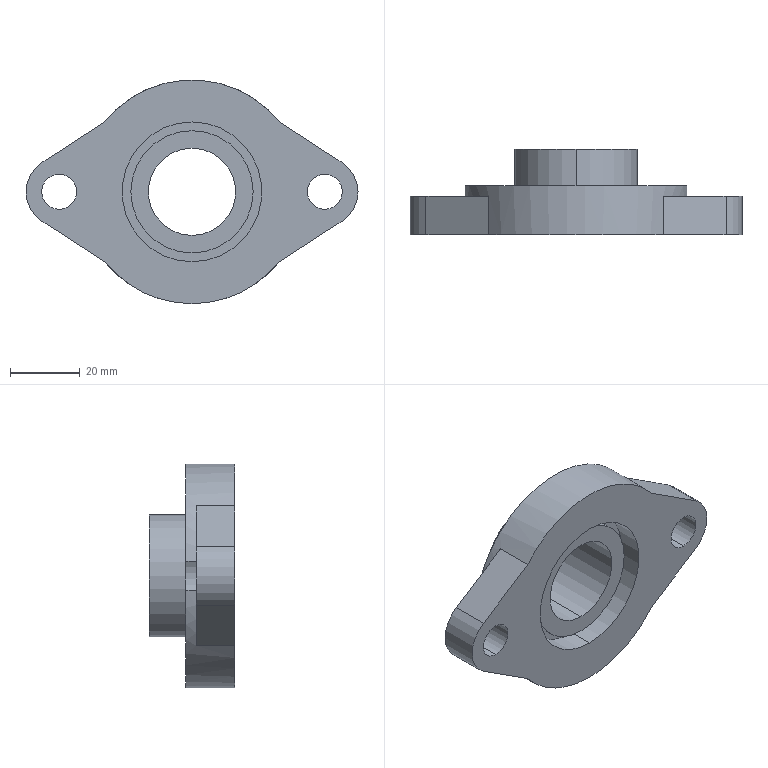Part | SolidWorks | features ICE 7, Extrusion 1, MirrorPattern 1 | 1 solid | 30 faces | box 95 x 24.5 x 64 mm | volume 45810 mm3 | cylinder 19 | plane 11 | commonest cylinder face diameters 10 x4 35 x4 64 x3 15 x2 20 x2 25 x2
STEP:
#1=CARTESIAN_POINT('',(0.,3.5,12.5));
#2=VERTEX_POINT('',#1);
#3=CARTESIAN_POINT('',(0.,3.5,-12.5));
#4=VERTEX_POINT('',#3);
#5=CARTESIAN_POINT('',(0.,3.5,0.));
#6=DIRECTION('',(0.,-1.,0.));
#7=DIRECTION('',(0.,0.,-1.));
#8=AXIS2_PLACEMENT_3D('',#5,#6,#7);
#9=CIRCLE('',#8,12.5);
#10=EDGE_CURVE('',#2,#4,#9,.T.);
#11=ORIENTED_EDGE('',*,*,#10,.T.);
#12=CARTESIAN_POINT('',(0.,24.5,-12.5));
#13=VERTEX_POINT('',#12);
#14=CARTESIAN_POINT('',(0.,0.,-12.5));
#15=DIRECTION('',(0.,1.,0.));
#16=VECTOR('',#15,1000.);
#17=LINE('',#14,#16);
#18=EDGE_CURVE('',#4,#13,#17,.T.);
#19=ORIENTED_EDGE('',*,*,#18,.T.);
#20=CARTESIAN_POINT('',(0.,24.5,12.5));
#21=VERTEX_POINT('',#20);
#22=CARTESIAN_POINT('',(0.,24.5,0.));
#23=DIRECTION('',(0.,1.,0.));
#24=DIRECTION('',(0.,0.,1.));
#25=AXIS2_PLACEMENT_3D('',#22,#23,#24);
#26=CIRCLE('',#25,12.5);
#27=EDGE_CURVE('',#13,#21,#26,.T.);
#28=ORIENTED_EDGE('',*,*,#27,.T.);
#29=CARTESIAN_POINT('',(0.,0.,12.5));
#30=DIRECTION('',(0.,1.,0.));
#31=VECTOR('',#30,1000.);
#32=LINE('',#29,#31);
#33=EDGE_CURVE('',#2,#21,#32,.T.);
#34=ORIENTED_EDGE('',*,*,#33,.F.);
#35=EDGE_LOOP('',(#11,#19,#28,#34));
#36=FACE_OUTER_BOUND('',#35,.T.);
#37=CARTESIAN_POINT('',(0.,0.,0.));
#38=DIRECTION('',(0.,1.,0.));
#39=DIRECTION('',(0.,0.,1.));
#40=AXIS2_PLACEMENT_3D('',#37,#38,#39);
#41=CYLINDRICAL_SURFACE('',#40,12.5);
#42=ADVANCED_FACE('',(#36),#41,.F.);
#43=CARTESIAN_POINT('',(0.,3.5,-17.5));
#44=VERTEX_POINT('',#43);
#45=CARTESIAN_POINT('',(0.,3.5,17.5));
#46=VERTEX_POINT('',#45);
#47=CARTESIAN_POINT('',(0.,3.5,0.));
#48=DIRECTION('',(0.,-1.,0.));
#49=DIRECTION('',(0.,0.,-1.));
#50=AXIS2_PLACEMENT_3D('',#47,#48,#49);
#51=CIRCLE('',#50,17.5);
#52=EDGE_CURVE('',#44,#46,#51,.T.);
#53=ORIENTED_EDGE('',*,*,#52,.F.);
#54=CARTESIAN_POINT('',(0.,7.,-17.5));
#55=VERTEX_POINT('',#54);
#56=CARTESIAN_POINT('',(0.,3.5,-17.5));
#57=DIRECTION('',(0.,1.,0.));
#58=VECTOR('',#57,1000.);
#59=LINE('',#56,#58);
#60=EDGE_CURVE('',#44,#55,#59,.T.);
#61=ORIENTED_EDGE('',*,*,#60,.T.);
#62=CARTESIAN_POINT('',(0.,7.,17.5));
#63=VERTEX_POINT('',#62);
#64=CARTESIAN_POINT('',(0.,7.,0.));
#65=DIRECTION('',(0.,-1.,0.));
#66=DIRECTION('',(0.,0.,-1.));
#67=AXIS2_PLACEMENT_3D('',#64,#65,#66);
#68=CIRCLE('',#67,17.5);
#69=EDGE_CURVE('',#55,#63,#68,.T.);
#70=ORIENTED_EDGE('',*,*,#69,.T.);
#71=CARTESIAN_POINT('',(0.,3.5,17.5));
#72=DIRECTION('',(0.,1.,0.));
#73=VECTOR('',#72,1000.);
#74=LINE('',#71,#73);
#75=EDGE_CURVE('',#46,#63,#74,.T.);
#76=ORIENTED_EDGE('',*,*,#75,.F.);
#77=EDGE_LOOP('',(#53,#61,#70,#76));
#78=FACE_OUTER_BOUND('',#77,.T.);
#79=CARTESIAN_POINT('',(0.,3.5,0.));
#80=DIRECTION('',(0.,1.,0.));
#81=DIRECTION('',(0.,0.,1.));
#82=AXIS2_PLACEMENT_3D('',#79,#80,#81);
#83=CYLINDRICAL_SURFACE('',#82,17.5);
#84=ADVANCED_FACE('',(#78),#83,.T.);
#85=CARTESIAN_POINT('',(0.,7.,20.));
#86=VERTEX_POINT('',#85);
#87=CARTESIAN_POINT('',(0.,7.,-20.));
#88=VERTEX_POINT('',#87);
#89=CARTESIAN_POINT('',(0.,7.,0.));
#90=DIRECTION('',(0.,-1.,0.));
#91=DIRECTION('',(0.,0.,-1.));
#92=AXIS2_PLACEMENT_3D('',#89,#90,#91);
#93=CIRCLE('',#92,20.);
#94=EDGE_CURVE('',#86,#88,#93,.T.);
#95=ORIENTED_EDGE('',*,*,#94,.F.);
#96=CARTESIAN_POINT('',(0.,0.,20.));
#97=VERTEX_POINT('',#96);
#98=CARTESIAN_POINT('',(0.,7.,20.));
#99=DIRECTION('',(0.,-1.,0.));
#100=VECTOR('',#99,1000.);
#101=LINE('',#98,#100);
#102=EDGE_CURVE('',#86,#97,#101,.T.);
#103=ORIENTED_EDGE('',*,*,#102,.T.);
#104=CARTESIAN_POINT('',(0.,0.,-20.));
#105=VERTEX_POINT('',#104);
#106=CARTESIAN_POINT('',(0.,0.,0.));
#107=DIRECTION('',(0.,-1.,0.));
#108=DIRECTION('',(0.,0.,-1.));
#109=AXIS2_PLACEMENT_3D('',#106,#107,#108);
#110=CIRCLE('',#109,20.);
#111=EDGE_CURVE('',#97,#105,#110,.T.);
#112=ORIENTED_EDGE('',*,*,#111,.T.);
#113=CARTESIAN_POINT('',(0.,7.,-20.));
#114=DIRECTION('',(0.,-1.,0.));
#115=VECTOR('',#114,1000.);
#116=LINE('',#113,#115);
#117=EDGE_CURVE('',#88,#105,#116,.T.);
#118=ORIENTED_EDGE('',*,*,#117,.F.);
#119=EDGE_LOOP('',(#95,#103,#112,#118));
#120=FACE_OUTER_BOUND('',#119,.T.);
#121=CARTESIAN_POINT('',(0.,7.,0.));
#122=DIRECTION('',(0.,-1.,0.));
#123=DIRECTION('',(0.,0.,-1.));
#124=AXIS2_PLACEMENT_3D('',#121,#122,#123);
#125=CYLINDRICAL_SURFACE('',#124,20.);
#126=ADVANCED_FACE('',(#120),#125,.F.);
#127=CARTESIAN_POINT('',(0.,24.5,17.5));
#128=VERTEX_POINT('',#127);
#129=CARTESIAN_POINT('',(0.,24.5,-17.5));
#130=VERTEX_POINT('',#129);
#131=CARTESIAN_POINT('',(0.,24.5,0.));
#132=DIRECTION('',(0.,1.,0.));
#133=DIRECTION('',(0.,0.,1.));
#134=AXIS2_PLACEMENT_3D('',#131,#132,#133);
#135=CIRCLE('',#134,17.5);
#136=EDGE_CURVE('',#128,#130,#135,.T.);
#137=ORIENTED_EDGE('',*,*,#136,.F.);
#138=CARTESIAN_POINT('',(0.,14.,17.5));
#139=VERTEX_POINT('',#138);
#140=CARTESIAN_POINT('',(0.,24.5,17.5));
#141=DIRECTION('',(0.,-1.,0.));
#142=VECTOR('',#141,1000.);
#143=LINE('',#140,#142);
#144=EDGE_CURVE('',#128,#139,#143,.T.);
#145=ORIENTED_EDGE('',*,*,#144,.T.);
#146=CARTESIAN_POINT('',(0.,14.,-17.5));
#147=VERTEX_POINT('',#146);
#148=CARTESIAN_POINT('',(0.,14.,0.));
#149=DIRECTION('',(0.,-1.,0.));
#150=DIRECTION('',(0.,0.,1.));
#151=AXIS2_PLACEMENT_3D('',#148,#149,#150);
#152=CIRCLE('',#151,17.5);
#153=EDGE_CURVE('',#147,#139,#152,.T.);
#154=ORIENTED_EDGE('',*,*,#153,.F.);
#155=CARTESIAN_POINT('',(0.,24.5,-17.5));
#156=DIRECTION('',(0.,-1.,0.));
#157=VECTOR('',#156,1000.);
#158=LINE('',#155,#157);
#159=EDGE_CURVE('',#130,#147,#158,.T.);
#160=ORIENTED_EDGE('',*,*,#159,.F.);
#161=EDGE_LOOP('',(#137,#145,#154,#160));
#162=FACE_OUTER_BOUND('',#161,.T.);
#163=CARTESIAN_POINT('',(0.,24.5,0.));
#164=DIRECTION('',(0.,-1.,0.));
#165=DIRECTION('',(0.,0.,-1.));
#166=AXIS2_PLACEMENT_3D('',#163,#164,#165);
#167=CYLINDRICAL_SURFACE('',#166,17.5);
#168=ADVANCED_FACE('',(#162),#167,.T.);
#169=CARTESIAN_POINT('',(38.,11.,5.));
#170=VERTEX_POINT('',#169);
#171=CARTESIAN_POINT('',(38.,11.,-5.));
#172=VERTEX_POINT('',#171);
#173=CARTESIAN_POINT('',(38.,11.,0.));
#174=DIRECTION('',(0.,-1.,0.));
#175=DIRECTION('',(0.,0.,1.));
#176=AXIS2_PLACEMENT_3D('',#173,#174,#175);
#177=CIRCLE('',#176,5.);
#178=EDGE_CURVE('',#170,#172,#177,.T.);
#179=ORIENTED_EDGE('',*,*,#178,.F.);
#180=CARTESIAN_POINT('',(38.,0.,5.));
#181=VERTEX_POINT('',#180);
#182=CARTESIAN_POINT('',(38.,14.,5.));
#183=DIRECTION('',(0.,-1.,0.));
#184=VECTOR('',#183,1000.);
#185=LINE('',#182,#184);
#186=EDGE_CURVE('',#170,#181,#185,.T.);
#187=ORIENTED_EDGE('',*,*,#186,.T.);
#188=CARTESIAN_POINT('',(38.,0.,-5.));
#189=VERTEX_POINT('',#188);
#190=CARTESIAN_POINT('',(38.,0.,0.));
#191=DIRECTION('',(0.,1.,0.));
#192=DIRECTION('',(0.,0.,1.));
#193=AXIS2_PLACEMENT_3D('',#190,#191,#192);
#194=CIRCLE('',#193,5.);
#195=EDGE_CURVE('',#189,#181,#194,.T.);
#196=ORIENTED_EDGE('',*,*,#195,.F.);
#197=CARTESIAN_POINT('',(38.,14.,-5.));
#198=DIRECTION('',(0.,-1.,0.));
#199=VECTOR('',#198,1000.);
#200=LINE('',#197,#199);
#201=EDGE_CURVE('',#172,#189,#200,.T.);
#202=ORIENTED_EDGE('',*,*,#201,.F.);
#203=EDGE_LOOP('',(#179,#187,#196,#202));
#204=FACE_OUTER_BOUND('',#203,.T.);
#205=CARTESIAN_POINT('',(38.,14.,0.));
#206=DIRECTION('',(0.,-1.,0.));
#207=DIRECTION('',(0.,0.,-1.));
#208=AXIS2_PLACEMENT_3D('',#205,#206,#207);
#209=CYLINDRICAL_SURFACE('',#208,5.);
#210=ADVANCED_FACE('',(#204),#209,.F.);
#211=CARTESIAN_POINT('',(-38.,11.,5.));
#212=VERTEX_POINT('',#211);
#213=CARTESIAN_POINT('',(-38.,11.,-5.));
#214=VERTEX_POINT('',#213);
#215=CARTESIAN_POINT('',(-38.,11.,0.));
#216=DIRECTION('',(0.,-1.,0.));
#217=DIRECTION('',(0.,0.,1.));
#218=AXIS2_PLACEMENT_3D('',#215,#216,#217);
#219=CIRCLE('',#218,5.);
#220=EDGE_CURVE('',#212,#214,#219,.T.);
#221=ORIENTED_EDGE('',*,*,#220,.F.);
#222=CARTESIAN_POINT('',(-38.,0.,5.));
#223=VERTEX_POINT('',#222);
#224=CARTESIAN_POINT('',(-38.,14.,5.));
#225=DIRECTION('',(0.,-1.,0.));
#226=VECTOR('',#225,1000.);
#227=LINE('',#224,#226);
#228=EDGE_CURVE('',#212,#223,#227,.T.);
#229=ORIENTED_EDGE('',*,*,#228,.T.);
#230=CARTESIAN_POINT('',(-38.,0.,-5.));
#231=VERTEX_POINT('',#230);
#232=CARTESIAN_POINT('',(-38.,0.,0.));
#233=DIRECTION('',(0.,1.,0.));
#234=DIRECTION('',(0.,0.,1.));
#235=AXIS2_PLACEMENT_3D('',#232,#233,#234);
#236=CIRCLE('',#235,5.);
#237=EDGE_CURVE('',#231,#223,#236,.T.);
#238=ORIENTED_EDGE('',*,*,#237,.F.);
#239=CARTESIAN_POINT('',(-38.,14.,-5.));
#240=DIRECTION('',(0.,-1.,0.));
#241=VECTOR('',#240,1000.);
#242=LINE('',#239,#241);
#243=EDGE_CURVE('',#214,#231,#242,.T.);
#244=ORIENTED_EDGE('',*,*,#243,.F.);
#245=EDGE_LOOP('',(#221,#229,#238,#244));
#246=FACE_OUTER_BOUND('',#245,.T.);
#247=CARTESIAN_POINT('',(-38.,14.,0.));
#248=DIRECTION('',(0.,-1.,0.));
#249=DIRECTION('',(0.,0.,-1.));
#250=AXIS2_PLACEMENT_3D('',#247,#248,#249);
#251=CYLINDRICAL_SURFACE('',#250,5.);
#252=ADVANCED_FACE('',(#246),#251,.F.);
#253=CARTESIAN_POINT('',(0.,14.,-32.));
#254=VERTEX_POINT('',#253);
#255=CARTESIAN_POINT('',(-31.734,14.,-4.121));
#256=VERTEX_POINT('',#255);
#257=CARTESIAN_POINT('',(0.,14.,0.));
#258=DIRECTION('',(0.,1.,0.));
#259=DIRECTION('',(0.,0.,1.));
#260=AXIS2_PLACEMENT_3D('',#257,#258,#259);
#261=CIRCLE('',#260,32.);
#262=EDGE_CURVE('',#254,#256,#261,.T.);
#263=ORIENTED_EDGE('',*,*,#262,.F.);
#264=CARTESIAN_POINT('',(0.,0.,-32.));
#265=VERTEX_POINT('',#264);
#266=CARTESIAN_POINT('',(0.,14.,-32.));
#267=DIRECTION('',(0.,-1.,0.));
#268=VECTOR('',#267,1000.);
#269=LINE('',#266,#268);
#270=EDGE_CURVE('',#254,#265,#269,.T.);
#271=ORIENTED_EDGE('',*,*,#270,.T.);
#272=CARTESIAN_POINT('',(-24.98,0.,-20.));
#273=VERTEX_POINT('',#272);
#274=CARTESIAN_POINT('',(0.,0.,0.));
#275=DIRECTION('',(0.,1.,0.));
#276=DIRECTION('',(0.,0.,1.));
#277=AXIS2_PLACEMENT_3D('',#274,#275,#276);
#278=CIRCLE('',#277,32.);
#279=EDGE_CURVE('',#265,#273,#278,.T.);
#280=ORIENTED_EDGE('',*,*,#279,.T.);
#281=CARTESIAN_POINT('',(-24.98,11.,-20.));
#282=VERTEX_POINT('',#281);
#283=CARTESIAN_POINT('',(-24.98,11.,-20.));
#284=DIRECTION('',(0.,-1.,0.));
#285=VECTOR('',#284,1000.);
#286=LINE('',#283,#285);
#287=EDGE_CURVE('',#282,#273,#286,.T.);
#288=ORIENTED_EDGE('',*,*,#287,.F.);
#289=CARTESIAN_POINT('',(-31.734,11.,-4.121));
#290=VERTEX_POINT('',#289);
#291=CARTESIAN_POINT('',(0.,11.,0.));
#292=DIRECTION('',(0.,1.,0.));
#293=DIRECTION('',(0.,0.,1.));
#294=AXIS2_PLACEMENT_3D('',#291,#292,#293);
#295=CIRCLE('',#294,32.);
#296=EDGE_CURVE('',#282,#290,#295,.T.);
#297=ORIENTED_EDGE('',*,*,#296,.T.);
#298=CARTESIAN_POINT('',(-31.734,12.5,-4.121));
#299=DIRECTION('',(0.,1.,0.));
#300=VECTOR('',#299,1000.);
#301=LINE('',#298,#300);
#302=EDGE_CURVE('',#290,#256,#301,.T.);
#303=ORIENTED_EDGE('',*,*,#302,.T.);
#304=EDGE_LOOP('',(#263,#271,#280,#288,#297,#303));
#305=FACE_OUTER_BOUND('',#304,.T.);
#306=CARTESIAN_POINT('',(0.,14.,0.));
#307=DIRECTION('',(0.,-1.,0.));
#308=DIRECTION('',(0.,0.,-1.));
#309=AXIS2_PLACEMENT_3D('',#306,#307,#308);
#310=CYLINDRICAL_SURFACE('',#309,32.);
#311=ADVANCED_FACE('',(#305),#310,.T.);
#312=CARTESIAN_POINT('',(0.,7.,0.));
#313=DIRECTION('',(0.,-1.,0.));
#314=DIRECTION('',(0.,0.,-1.));
#315=AXIS2_PLACEMENT_3D('',#312,#313,#314);
#316=CIRCLE('',#315,20.);
#317=EDGE_CURVE('',#88,#86,#316,.T.);
#318=ORIENTED_EDGE('',*,*,#317,.T.);
#319=ORIENTED_EDGE('',*,*,#94,.T.);
#320=EDGE_LOOP('',(#318,#319));
#321=FACE_OUTER_BOUND('',#320,.T.);
#322=CARTESIAN_POINT('',(0.,7.,0.));
#323=DIRECTION('',(0.,-1.,0.));
#324=DIRECTION('',(0.,0.,-1.));
#325=AXIS2_PLACEMENT_3D('',#322,#323,#324);
#326=CIRCLE('',#325,17.5);
#327=EDGE_CURVE('',#63,#55,#326,.T.);
#328=ORIENTED_EDGE('',*,*,#327,.F.);
#329=ORIENTED_EDGE('',*,*,#69,.F.);
#330=EDGE_LOOP('',(#328,#329));
#331=FACE_BOUND('',#330,.T.);
#332=CARTESIAN_POINT('',(0.,7.,0.));
#333=DIRECTION('',(0.,-1.,0.));
#334=DIRECTION('',(0.,0.,-1.));
#335=AXIS2_PLACEMENT_3D('',#332,#333,#334);
#336=PLANE('',#335);
#337=ADVANCED_FACE('',(#321,#331),#336,.T.);
#338=CARTESIAN_POINT('',(31.734,14.,-4.121));
#339=VERTEX_POINT('',#338);
#340=CARTESIAN_POINT('',(31.734,14.,4.121));
#341=VERTEX_POINT('',#340);
#342=CARTESIAN_POINT('',(38.,14.,0.));
#343=DIRECTION('',(0.,1.,0.));
#344=DIRECTION('',(0.,0.,1.));
#345=AXIS2_PLACEMENT_3D('',#342,#343,#344);
#346=CIRCLE('',#345,7.5);
#347=EDGE_CURVE('',#339,#341,#346,.T.);
#348=ORIENTED_EDGE('',*,*,#347,.F.);
#349=CARTESIAN_POINT('',(0.,14.,0.));
#350=DIRECTION('',(0.,1.,0.));
#351=DIRECTION('',(0.,0.,1.));
#352=AXIS2_PLACEMENT_3D('',#349,#350,#351);
#353=CIRCLE('',#352,32.);
#354=EDGE_CURVE('',#339,#254,#353,.T.);
#355=ORIENTED_EDGE('',*,*,#354,.T.);
#356=ORIENTED_EDGE('',*,*,#262,.T.);
#357=CARTESIAN_POINT('',(-31.734,14.,4.121));
#358=VERTEX_POINT('',#357);
#359=CARTESIAN_POINT('',(-38.,14.,0.));
#360=DIRECTION('',(0.,1.,0.));
#361=DIRECTION('',(0.,0.,1.));
#362=AXIS2_PLACEMENT_3D('',#359,#360,#361);
#363=CIRCLE('',#362,7.5);
#364=EDGE_CURVE('',#358,#256,#363,.T.);
#365=ORIENTED_EDGE('',*,*,#364,.F.);
#366=CARTESIAN_POINT('',(0.,14.,0.));
#367=DIRECTION('',(0.,1.,0.));
#368=DIRECTION('',(0.,0.,1.));
#369=AXIS2_PLACEMENT_3D('',#366,#367,#368);
#370=CIRCLE('',#369,32.);
#371=EDGE_CURVE('',#358,#341,#370,.T.);
#372=ORIENTED_EDGE('',*,*,#371,.T.);
#373=EDGE_LOOP('',(#348,#355,#356,#365,#372));
#374=FACE_OUTER_BOUND('',#373,.T.);
#375=ORIENTED_EDGE('',*,*,#153,.T.);
#376=CARTESIAN_POINT('',(0.,14.,0.));
#377=DIRECTION('',(0.,-1.,0.));
#378=DIRECTION('',(0.,0.,1.));
#379=AXIS2_PLACEMENT_3D('',#376,#377,#378);
#380=CIRCLE('',#379,17.5);
#381=EDGE_CURVE('',#139,#147,#380,.T.);
#382=ORIENTED_EDGE('',*,*,#381,.T.);
#383=EDGE_LOOP('',(#375,#382));
#384=FACE_BOUND('',#383,.T.);
#385=CARTESIAN_POINT('',(0.,14.,0.));
#386=DIRECTION('',(0.,1.,0.));
#387=DIRECTION('',(0.,0.,1.));
#388=AXIS2_PLACEMENT_3D('',#385,#386,#387);
#389=PLANE('',#388);
#390=ADVANCED_FACE('',(#374,#384),#389,.T.);
#391=CARTESIAN_POINT('',(31.734,11.,4.121));
#392=VERTEX_POINT('',#391);
#393=CARTESIAN_POINT('',(24.98,11.,20.));
#394=VERTEX_POINT('',#393);
#395=CARTESIAN_POINT('',(0.,11.,0.));
#396=DIRECTION('',(0.,-1.,0.));
#397=DIRECTION('',(0.,0.,1.));
#398=AXIS2_PLACEMENT_3D('',#395,#396,#397);
#399=CIRCLE('',#398,32.);
#400=EDGE_CURVE('',#392,#394,#399,.T.);
#401=ORIENTED_EDGE('',*,*,#400,.F.);
#402=CARTESIAN_POINT('',(31.734,12.5,4.121));
#403=DIRECTION('',(0.,1.,0.));
#404=VECTOR('',#403,1000.);
#405=LINE('',#402,#404);
#406=EDGE_CURVE('',#392,#341,#405,.T.);
#407=ORIENTED_EDGE('',*,*,#406,.T.);
#408=ORIENTED_EDGE('',*,*,#371,.F.);
#409=CARTESIAN_POINT('',(-31.734,11.,4.121));
#410=VERTEX_POINT('',#409);
#411=CARTESIAN_POINT('',(-31.734,12.5,4.121));
#412=DIRECTION('',(0.,-1.,0.));
#413=VECTOR('',#412,1000.);
#414=LINE('',#411,#413);
#415=EDGE_CURVE('',#358,#410,#414,.T.);
#416=ORIENTED_EDGE('',*,*,#415,.T.);
#417=CARTESIAN_POINT('',(-24.98,11.,20.));
#418=VERTEX_POINT('',#417);
#419=CARTESIAN_POINT('',(0.,11.,0.));
#420=DIRECTION('',(0.,1.,0.));
#421=DIRECTION('',(0.,0.,1.));
#422=AXIS2_PLACEMENT_3D('',#419,#420,#421);
#423=CIRCLE('',#422,32.);
#424=EDGE_CURVE('',#410,#418,#423,.T.);
#425=ORIENTED_EDGE('',*,*,#424,.T.);
#426=CARTESIAN_POINT('',(-24.98,0.,20.));
#427=VERTEX_POINT('',#426);
#428=CARTESIAN_POINT('',(-24.98,11.,20.));
#429=DIRECTION('',(0.,-1.,0.));
#430=VECTOR('',#429,1000.);
#431=LINE('',#428,#430);
#432=EDGE_CURVE('',#418,#427,#431,.T.);
#433=ORIENTED_EDGE('',*,*,#432,.T.);
#434=CARTESIAN_POINT('',(24.98,0.,20.));
#435=VERTEX_POINT('',#434);
#436=CARTESIAN_POINT('',(0.,0.,0.));
#437=DIRECTION('',(0.,1.,0.));
#438=DIRECTION('',(0.,0.,1.));
#439=AXIS2_PLACEMENT_3D('',#436,#437,#438);
#440=CIRCLE('',#439,32.);
#441=EDGE_CURVE('',#427,#435,#440,.T.);
#442=ORIENTED_EDGE('',*,*,#441,.T.);
#443=CARTESIAN_POINT('',(24.98,11.,20.));
#444=DIRECTION('',(0.,-1.,0.));
#445=VECTOR('',#444,1000.);
#446=LINE('',#443,#445);
#447=EDGE_CURVE('',#394,#435,#446,.T.);
#448=ORIENTED_EDGE('',*,*,#447,.F.);
#449=EDGE_LOOP('',(#401,#407,#408,#416,#425,#433,#442,#448));
#450=FACE_OUTER_BOUND('',#449,.T.);
#451=CARTESIAN_POINT('',(0.,14.,0.));
#452=DIRECTION('',(0.,-1.,0.));
#453=DIRECTION('',(0.,0.,-1.));
#454=AXIS2_PLACEMENT_3D('',#451,#452,#453);
#455=CYLINDRICAL_SURFACE('',#454,32.);
#456=ADVANCED_FACE('',(#450),#455,.T.);
#457=CARTESIAN_POINT('',(0.,0.,0.));
#458=DIRECTION('',(0.,-1.,0.));
#459=DIRECTION('',(0.,0.,-1.));
#460=AXIS2_PLACEMENT_3D('',#457,#458,#459);
#461=CIRCLE('',#460,20.);
#462=EDGE_CURVE('',#105,#97,#461,.T.);
#463=ORIENTED_EDGE('',*,*,#462,.F.);
#464=ORIENTED_EDGE('',*,*,#111,.F.);
#465=EDGE_LOOP('',(#463,#464));
#466=FACE_BOUND('',#465,.T.);
#467=ORIENTED_EDGE('',*,*,#195,.T.);
#468=CARTESIAN_POINT('',(38.,0.,0.));
#469=DIRECTION('',(0.,1.,0.));
#470=DIRECTION('',(0.,0.,1.));
#471=AXIS2_PLACEMENT_3D('',#468,#469,#470);
#472=CIRCLE('',#471,5.);
#473=EDGE_CURVE('',#181,#189,#472,.T.);
#474=ORIENTED_EDGE('',*,*,#473,.T.);
#475=EDGE_LOOP('',(#467,#474));
#476=FACE_BOUND('',#475,.T.);
#477=CARTESIAN_POINT('',(24.98,0.,-20.));
#478=VERTEX_POINT('',#477);
#479=CARTESIAN_POINT('',(0.,0.,0.));
#480=DIRECTION('',(0.,1.,0.));
#481=DIRECTION('',(0.,0.,1.));
#482=AXIS2_PLACEMENT_3D('',#479,#480,#481);
#483=CIRCLE('',#482,32.);
#484=EDGE_CURVE('',#478,#265,#483,.T.);
#485=ORIENTED_EDGE('',*,*,#484,.F.);
#486=CARTESIAN_POINT('',(42.929,0.,-8.398));
#487=VERTEX_POINT('',#486);
#488=CARTESIAN_POINT('',(42.929,0.,-8.398));
#489=DIRECTION('',(-0.8398,0.,-0.5429));
#490=VECTOR('',#489,1000.);
#491=LINE('',#488,#490);
#492=EDGE_CURVE('',#487,#478,#491,.T.);
#493=ORIENTED_EDGE('',*,*,#492,.F.);
#494=CARTESIAN_POINT('',(42.929,0.,8.398));
#495=VERTEX_POINT('',#494);
#496=CARTESIAN_POINT('',(37.5,0.,0.));
#497=DIRECTION('',(0.,1.,0.));
#498=DIRECTION('',(0.,0.,1.));
#499=AXIS2_PLACEMENT_3D('',#496,#497,#498);
#500=CIRCLE('',#499,10.);
#501=EDGE_CURVE('',#495,#487,#500,.T.);
#502=ORIENTED_EDGE('',*,*,#501,.F.);
#503=CARTESIAN_POINT('',(42.929,0.,8.398));
#504=DIRECTION('',(0.8398,0.,-0.5429));
#505=VECTOR('',#504,1000.);
#506=LINE('',#503,#505);
#507=EDGE_CURVE('',#435,#495,#506,.T.);
#508=ORIENTED_EDGE('',*,*,#507,.F.);
#509=ORIENTED_EDGE('',*,*,#441,.F.);
#510=CARTESIAN_POINT('',(-42.929,0.,8.398));
#511=VERTEX_POINT('',#510);
#512=CARTESIAN_POINT('',(-42.929,0.,8.398));
#513=DIRECTION('',(-0.8398,0.,-0.5429));
#514=VECTOR('',#513,1000.);
#515=LINE('',#512,#514);
#516=EDGE_CURVE('',#427,#511,#515,.T.);
#517=ORIENTED_EDGE('',*,*,#516,.T.);
#518=CARTESIAN_POINT('',(-42.929,0.,-8.398));
#519=VERTEX_POINT('',#518);
#520=CARTESIAN_POINT('',(-37.5,0.,0.));
#521=DIRECTION('',(0.,-1.,0.));
#522=DIRECTION('',(0.,0.,1.));
#523=AXIS2_PLACEMENT_3D('',#520,#521,#522);
#524=CIRCLE('',#523,10.);
#525=EDGE_CURVE('',#511,#519,#524,.T.);
#526=ORIENTED_EDGE('',*,*,#525,.T.);
#527=CARTESIAN_POINT('',(-42.929,0.,-8.398));
#528=DIRECTION('',(0.8398,0.,-0.5429));
#529=VECTOR('',#528,1000.);
#530=LINE('',#527,#529);
#531=EDGE_CURVE('',#519,#273,#530,.T.);
#532=ORIENTED_EDGE('',*,*,#531,.T.);
#533=ORIENTED_EDGE('',*,*,#279,.F.);
#534=EDGE_LOOP('',(#485,#493,#502,#508,#509,#517,#526,#532,#533));
#535=FACE_OUTER_BOUND('',#534,.T.);
#536=ORIENTED_EDGE('',*,*,#237,.T.);
#537=CARTESIAN_POINT('',(-38.,0.,0.));
#538=DIRECTION('',(0.,1.,0.));
#539=DIRECTION('',(0.,0.,1.));
#540=AXIS2_PLACEMENT_3D('',#537,#538,#539);
#541=CIRCLE('',#540,5.);
#542=EDGE_CURVE('',#223,#231,#541,.T.);
#543=ORIENTED_EDGE('',*,*,#542,.T.);
#544=EDGE_LOOP('',(#536,#543));
#545=FACE_BOUND('',#544,.T.);
#546=CARTESIAN_POINT('',(0.,0.,0.));
#547=DIRECTION('',(0.,1.,0.));
#548=DIRECTION('',(0.,0.,1.));
#549=AXIS2_PLACEMENT_3D('',#546,#547,#548);
#550=PLANE('',#549);
#551=ADVANCED_FACE('',(#466,#476,#535,#545),#550,.F.);
#552=CARTESIAN_POINT('',(24.98,11.,-20.));
#553=VERTEX_POINT('',#552);
#554=CARTESIAN_POINT('',(31.734,11.,-4.121));
#555=VERTEX_POINT('',#554);
#556=CARTESIAN_POINT('',(0.,11.,0.));
#557=DIRECTION('',(0.,-1.,0.));
#558=DIRECTION('',(0.,0.,1.));
#559=AXIS2_PLACEMENT_3D('',#556,#557,#558);
#560=CIRCLE('',#559,32.);
#561=EDGE_CURVE('',#553,#555,#560,.T.);
#562=ORIENTED_EDGE('',*,*,#561,.T.);
#563=CARTESIAN_POINT('',(38.,11.,0.));
#564=DIRECTION('',(0.,-1.,0.));
#565=DIRECTION('',(0.,0.,1.));
#566=AXIS2_PLACEMENT_3D('',#563,#564,#565);
#567=CIRCLE('',#566,7.5);
#568=EDGE_CURVE('',#392,#555,#567,.T.);
#569=ORIENTED_EDGE('',*,*,#568,.F.);
#570=ORIENTED_EDGE('',*,*,#400,.T.);
#571=CARTESIAN_POINT('',(42.929,11.,8.398));
#572=VERTEX_POINT('',#571);
#573=CARTESIAN_POINT('',(42.929,11.,8.398));
#574=DIRECTION('',(0.8398,0.,-0.5429));
#575=VECTOR('',#574,1000.);
#576=LINE('',#573,#575);
#577=EDGE_CURVE('',#394,#572,#576,.T.);
#578=ORIENTED_EDGE('',*,*,#577,.T.);
#579=CARTESIAN_POINT('',(42.929,11.,-8.398));
#580=VERTEX_POINT('',#579);
#581=CARTESIAN_POINT('',(37.5,11.,0.));
#582=DIRECTION('',(0.,1.,0.));
#583=DIRECTION('',(0.,0.,1.));
#584=AXIS2_PLACEMENT_3D('',#581,#582,#583);
#585=CIRCLE('',#584,10.);
#586=EDGE_CURVE('',#572,#580,#585,.T.);
#587=ORIENTED_EDGE('',*,*,#586,.T.);
#588=CARTESIAN_POINT('',(42.929,11.,-8.398));
#589=DIRECTION('',(-0.8398,0.,-0.5429));
#590=VECTOR('',#589,1000.);
#591=LINE('',#588,#590);
#592=EDGE_CURVE('',#580,#553,#591,.T.);
#593=ORIENTED_EDGE('',*,*,#592,.T.);
#594=EDGE_LOOP('',(#562,#569,#570,#578,#587,#593));
#595=FACE_OUTER_BOUND('',#594,.T.);
#596=CARTESIAN_POINT('',(38.,11.,0.));
#597=DIRECTION('',(0.,-1.,0.));
#598=DIRECTION('',(0.,0.,1.));
#599=AXIS2_PLACEMENT_3D('',#596,#597,#598);
#600=CIRCLE('',#599,5.);
#601=EDGE_CURVE('',#172,#170,#600,.T.);
#602=ORIENTED_EDGE('',*,*,#601,.T.);
#603=ORIENTED_EDGE('',*,*,#178,.T.);
#604=EDGE_LOOP('',(#602,#603));
#605=FACE_BOUND('',#604,.T.);
#606=CARTESIAN_POINT('',(37.5,11.,0.));
#607=DIRECTION('',(0.,1.,0.));
#608=DIRECTION('',(0.,0.,1.));
#609=AXIS2_PLACEMENT_3D('',#606,#607,#608);
#610=PLANE('',#609);
#611=ADVANCED_FACE('',(#595,#605),#610,.T.);
#612=ORIENTED_EDGE('',*,*,#424,.F.);
#613=CARTESIAN_POINT('',(-38.,11.,0.));
#614=DIRECTION('',(0.,-1.,0.));
#615=DIRECTION('',(0.,0.,1.));
#616=AXIS2_PLACEMENT_3D('',#613,#614,#615);
#617=CIRCLE('',#616,7.5);
#618=EDGE_CURVE('',#290,#410,#617,.T.);
#619=ORIENTED_EDGE('',*,*,#618,.F.);
#620=ORIENTED_EDGE('',*,*,#296,.F.);
#621=CARTESIAN_POINT('',(-42.929,11.,-8.398));
#622=VERTEX_POINT('',#621);
#623=CARTESIAN_POINT('',(-42.929,11.,-8.398));
#624=DIRECTION('',(0.8398,0.,-0.5429));
#625=VECTOR('',#624,1000.);
#626=LINE('',#623,#625);
#627=EDGE_CURVE('',#622,#282,#626,.T.);
#628=ORIENTED_EDGE('',*,*,#627,.F.);
#629=CARTESIAN_POINT('',(-42.929,11.,8.398));
#630=VERTEX_POINT('',#629);
#631=CARTESIAN_POINT('',(-37.5,11.,0.));
#632=DIRECTION('',(0.,-1.,0.));
#633=DIRECTION('',(0.,0.,1.));
#634=AXIS2_PLACEMENT_3D('',#631,#632,#633);
#635=CIRCLE('',#634,10.);
#636=EDGE_CURVE('',#630,#622,#635,.T.);
#637=ORIENTED_EDGE('',*,*,#636,.F.);
#638=CARTESIAN_POINT('',(-42.929,11.,8.398));
#639=DIRECTION('',(-0.8398,0.,-0.5429));
#640=VECTOR('',#639,1000.);
#641=LINE('',#638,#640);
#642=EDGE_CURVE('',#418,#630,#641,.T.);
#643=ORIENTED_EDGE('',*,*,#642,.F.);
#644=EDGE_LOOP('',(#612,#619,#620,#628,#637,#643));
#645=FACE_OUTER_BOUND('',#644,.T.);
#646=CARTESIAN_POINT('',(-38.,11.,0.));
#647=DIRECTION('',(0.,-1.,0.));
#648=DIRECTION('',(0.,0.,1.));
#649=AXIS2_PLACEMENT_3D('',#646,#647,#648);
#650=CIRCLE('',#649,5.);
#651=EDGE_CURVE('',#214,#212,#650,.T.);
#652=ORIENTED_EDGE('',*,*,#651,.T.);
#653=ORIENTED_EDGE('',*,*,#220,.T.);
#654=EDGE_LOOP('',(#652,#653));
#655=FACE_BOUND('',#654,.T.);
#656=CARTESIAN_POINT('',(-37.5,11.,0.));
#657=DIRECTION('',(0.,1.,0.));
#658=DIRECTION('',(0.,0.,1.));
#659=AXIS2_PLACEMENT_3D('',#656,#657,#658);
#660=PLANE('',#659);
#661=ADVANCED_FACE('',(#645,#655),#660,.T.);
#662=ORIENTED_EDGE('',*,*,#270,.F.);
#663=ORIENTED_EDGE('',*,*,#354,.F.);
#664=CARTESIAN_POINT('',(31.734,12.5,-4.121));
#665=DIRECTION('',(0.,-1.,0.));
#666=VECTOR('',#665,1000.);
#667=LINE('',#664,#666);
#668=EDGE_CURVE('',#339,#555,#667,.T.);
#669=ORIENTED_EDGE('',*,*,#668,.T.);
#670=ORIENTED_EDGE('',*,*,#561,.F.);
#671=CARTESIAN_POINT('',(24.98,11.,-20.));
#672=DIRECTION('',(0.,-1.,0.));
#673=VECTOR('',#672,1000.);
#674=LINE('',#671,#673);
#675=EDGE_CURVE('',#553,#478,#674,.T.);
#676=ORIENTED_EDGE('',*,*,#675,.T.);
#677=ORIENTED_EDGE('',*,*,#484,.T.);
#678=EDGE_LOOP('',(#662,#663,#669,#670,#676,#677));
#679=FACE_OUTER_BOUND('',#678,.T.);
#680=CARTESIAN_POINT('',(0.,14.,0.));
#681=DIRECTION('',(0.,-1.,0.));
#682=DIRECTION('',(0.,0.,-1.));
#683=AXIS2_PLACEMENT_3D('',#680,#681,#682);
#684=CYLINDRICAL_SURFACE('',#683,32.);
#685=ADVANCED_FACE('',(#679),#684,.T.);
#686=ORIENTED_EDGE('',*,*,#501,.T.);
#687=CARTESIAN_POINT('',(42.929,11.,-8.398));
#688=DIRECTION('',(0.,-1.,0.));
#689=VECTOR('',#688,1000.);
#690=LINE('',#687,#689);
#691=EDGE_CURVE('',#580,#487,#690,.T.);
#692=ORIENTED_EDGE('',*,*,#691,.F.);
#693=ORIENTED_EDGE('',*,*,#586,.F.);
#694=CARTESIAN_POINT('',(42.929,11.,8.398));
#695=DIRECTION('',(0.,-1.,0.));
#696=VECTOR('',#695,1000.);
#697=LINE('',#694,#696);
#698=EDGE_CURVE('',#572,#495,#697,.T.);
#699=ORIENTED_EDGE('',*,*,#698,.T.);
#700=EDGE_LOOP('',(#686,#692,#693,#699));
#701=FACE_OUTER_BOUND('',#700,.T.);
#702=CARTESIAN_POINT('',(37.5,11.,0.));
#703=DIRECTION('',(0.,-1.,0.));
#704=DIRECTION('',(0.,0.,-1.));
#705=AXIS2_PLACEMENT_3D('',#702,#703,#704);
#706=CYLINDRICAL_SURFACE('',#705,10.);
#707=ADVANCED_FACE('',(#701),#706,.T.);
#708=ORIENTED_EDGE('',*,*,#492,.T.);
#709=ORIENTED_EDGE('',*,*,#675,.F.);
#710=ORIENTED_EDGE('',*,*,#592,.F.);
#711=ORIENTED_EDGE('',*,*,#691,.T.);
#712=EDGE_LOOP('',(#708,#709,#710,#711));
#713=FACE_OUTER_BOUND('',#712,.T.);
#714=CARTESIAN_POINT('',(42.929,11.,-8.398));
#715=DIRECTION('',(-0.5429,0.,0.8398));
#716=DIRECTION('',(0.8398,0.,0.5429));
#717=AXIS2_PLACEMENT_3D('',#714,#715,#716);
#718=PLANE('',#717);
#719=ADVANCED_FACE('',(#713),#718,.F.);
#720=ORIENTED_EDGE('',*,*,#507,.T.);
#721=ORIENTED_EDGE('',*,*,#698,.F.);
#722=ORIENTED_EDGE('',*,*,#577,.F.);
#723=ORIENTED_EDGE('',*,*,#447,.T.);
#724=EDGE_LOOP('',(#720,#721,#722,#723));
#725=FACE_OUTER_BOUND('',#724,.T.);
#726=CARTESIAN_POINT('',(42.929,11.,8.398));
#727=DIRECTION('',(-0.5429,0.,-0.8398));
#728=DIRECTION('',(-0.8398,0.,0.5429));
#729=AXIS2_PLACEMENT_3D('',#726,#727,#728);
#730=PLANE('',#729);
#731=ADVANCED_FACE('',(#725),#730,.F.);
#732=ORIENTED_EDGE('',*,*,#525,.F.);
#733=CARTESIAN_POINT('',(-42.929,11.,8.398));
#734=DIRECTION('',(0.,-1.,0.));
#735=VECTOR('',#734,1000.);
#736=LINE('',#733,#735);
#737=EDGE_CURVE('',#630,#511,#736,.T.);
#738=ORIENTED_EDGE('',*,*,#737,.F.);
#739=ORIENTED_EDGE('',*,*,#636,.T.);
#740=CARTESIAN_POINT('',(-42.929,11.,-8.398));
#741=DIRECTION('',(0.,-1.,0.));
#742=VECTOR('',#741,1000.);
#743=LINE('',#740,#742);
#744=EDGE_CURVE('',#622,#519,#743,.T.);
#745=ORIENTED_EDGE('',*,*,#744,.T.);
#746=EDGE_LOOP('',(#732,#738,#739,#745));
#747=FACE_OUTER_BOUND('',#746,.T.);
#748=CARTESIAN_POINT('',(-37.5,11.,0.));
#749=DIRECTION('',(0.,-1.,0.));
#750=DIRECTION('',(0.,0.,-1.));
#751=AXIS2_PLACEMENT_3D('',#748,#749,#750);
#752=CYLINDRICAL_SURFACE('',#751,10.);
#753=ADVANCED_FACE('',(#747),#752,.T.);
#754=ORIENTED_EDGE('',*,*,#516,.F.);
#755=ORIENTED_EDGE('',*,*,#432,.F.);
#756=ORIENTED_EDGE('',*,*,#642,.T.);
#757=ORIENTED_EDGE('',*,*,#737,.T.);
#758=EDGE_LOOP('',(#754,#755,#756,#757));
#759=FACE_OUTER_BOUND('',#758,.T.);
#760=CARTESIAN_POINT('',(-42.929,11.,8.398));
#761=DIRECTION('',(-0.5429,0.,0.8398));
#762=DIRECTION('',(0.8398,0.,0.5429));
#763=AXIS2_PLACEMENT_3D('',#760,#761,#762);
#764=PLANE('',#763);
#765=ADVANCED_FACE('',(#759),#764,.T.);
#766=ORIENTED_EDGE('',*,*,#531,.F.);
#767=ORIENTED_EDGE('',*,*,#744,.F.);
#768=ORIENTED_EDGE('',*,*,#627,.T.);
#769=ORIENTED_EDGE('',*,*,#287,.T.);
#770=EDGE_LOOP('',(#766,#767,#768,#769));
#771=FACE_OUTER_BOUND('',#770,.T.);
#772=CARTESIAN_POINT('',(-42.929,11.,-8.398));
#773=DIRECTION('',(-0.5429,0.,-0.8398));
#774=DIRECTION('',(-0.8398,0.,0.5429));
#775=AXIS2_PLACEMENT_3D('',#772,#773,#774);
#776=PLANE('',#775);
#777=ADVANCED_FACE('',(#771),#776,.T.);
#778=ORIENTED_EDGE('',*,*,#228,.F.);
#779=ORIENTED_EDGE('',*,*,#651,.F.);
#780=ORIENTED_EDGE('',*,*,#243,.T.);
#781=ORIENTED_EDGE('',*,*,#542,.F.);
#782=EDGE_LOOP('',(#778,#779,#780,#781));
#783=FACE_OUTER_BOUND('',#782,.T.);
#784=CARTESIAN_POINT('',(-38.,14.,0.));
#785=DIRECTION('',(0.,-1.,0.));
#786=DIRECTION('',(0.,0.,-1.));
#787=AXIS2_PLACEMENT_3D('',#784,#785,#786);
#788=CYLINDRICAL_SURFACE('',#787,5.);
#789=ADVANCED_FACE('',(#783),#788,.F.);
#790=ORIENTED_EDGE('',*,*,#186,.F.);
#791=ORIENTED_EDGE('',*,*,#601,.F.);
#792=ORIENTED_EDGE('',*,*,#201,.T.);
#793=ORIENTED_EDGE('',*,*,#473,.F.);
#794=EDGE_LOOP('',(#790,#791,#792,#793));
#795=FACE_OUTER_BOUND('',#794,.T.);
#796=CARTESIAN_POINT('',(38.,14.,0.));
#797=DIRECTION('',(0.,-1.,0.));
#798=DIRECTION('',(0.,0.,-1.));
#799=AXIS2_PLACEMENT_3D('',#796,#797,#798);
#800=CYLINDRICAL_SURFACE('',#799,5.);
#801=ADVANCED_FACE('',(#795),#800,.F.);
#802=ORIENTED_EDGE('',*,*,#618,.T.);
#803=ORIENTED_EDGE('',*,*,#415,.F.);
#804=ORIENTED_EDGE('',*,*,#364,.T.);
#805=ORIENTED_EDGE('',*,*,#302,.F.);
#806=EDGE_LOOP('',(#802,#803,#804,#805));
#807=FACE_OUTER_BOUND('',#806,.T.);
#808=CARTESIAN_POINT('',(-38.,-10.213,0.));
#809=DIRECTION('',(0.,1.,0.));
#810=DIRECTION('',(0.,0.,1.));
#811=AXIS2_PLACEMENT_3D('',#808,#809,#810);
#812=CYLINDRICAL_SURFACE('',#811,7.5);
#813=ADVANCED_FACE('',(#807),#812,.F.);
#814=ORIENTED_EDGE('',*,*,#568,.T.);
#815=ORIENTED_EDGE('',*,*,#668,.F.);
#816=ORIENTED_EDGE('',*,*,#347,.T.);
#817=ORIENTED_EDGE('',*,*,#406,.F.);
#818=EDGE_LOOP('',(#814,#815,#816,#817));
#819=FACE_OUTER_BOUND('',#818,.T.);
#820=CARTESIAN_POINT('',(38.,-10.213,0.));
#821=DIRECTION('',(0.,1.,0.));
#822=DIRECTION('',(0.,0.,1.));
#823=AXIS2_PLACEMENT_3D('',#820,#821,#822);
#824=CYLINDRICAL_SURFACE('',#823,7.5);
#825=ADVANCED_FACE('',(#819),#824,.F.);
#826=ORIENTED_EDGE('',*,*,#144,.F.);
#827=CARTESIAN_POINT('',(0.,24.5,0.));
#828=DIRECTION('',(0.,1.,0.));
#829=DIRECTION('',(0.,0.,1.));
#830=AXIS2_PLACEMENT_3D('',#827,#828,#829);
#831=CIRCLE('',#830,17.5);
#832=EDGE_CURVE('',#130,#128,#831,.T.);
#833=ORIENTED_EDGE('',*,*,#832,.F.);
#834=ORIENTED_EDGE('',*,*,#159,.T.);
#835=ORIENTED_EDGE('',*,*,#381,.F.);
#836=EDGE_LOOP('',(#826,#833,#834,#835));
#837=FACE_OUTER_BOUND('',#836,.T.);
#838=CARTESIAN_POINT('',(0.,24.5,0.));
#839=DIRECTION('',(0.,-1.,0.));
#840=DIRECTION('',(0.,0.,-1.));
#841=AXIS2_PLACEMENT_3D('',#838,#839,#840);
#842=CYLINDRICAL_SURFACE('',#841,17.5);
#843=ADVANCED_FACE('',(#837),#842,.T.);
#844=CARTESIAN_POINT('',(0.,24.5,0.));
#845=DIRECTION('',(0.,1.,0.));
#846=DIRECTION('',(0.,0.,1.));
#847=AXIS2_PLACEMENT_3D('',#844,#845,#846);
#848=CIRCLE('',#847,12.5);
#849=EDGE_CURVE('',#21,#13,#848,.T.);
#850=ORIENTED_EDGE('',*,*,#849,.F.);
#851=ORIENTED_EDGE('',*,*,#27,.F.);
#852=EDGE_LOOP('',(#850,#851));
#853=FACE_BOUND('',#852,.T.);
#854=ORIENTED_EDGE('',*,*,#832,.T.);
#855=ORIENTED_EDGE('',*,*,#136,.T.);
#856=EDGE_LOOP('',(#854,#855));
#857=FACE_OUTER_BOUND('',#856,.T.);
#858=CARTESIAN_POINT('',(0.,24.5,0.));
#859=DIRECTION('',(0.,1.,0.));
#860=DIRECTION('',(0.,0.,1.));
#861=AXIS2_PLACEMENT_3D('',#858,#859,#860);
#862=PLANE('',#861);
#863=ADVANCED_FACE('',(#853,#857),#862,.T.);
#864=ORIENTED_EDGE('',*,*,#102,.F.);
#865=ORIENTED_EDGE('',*,*,#317,.F.);
#866=ORIENTED_EDGE('',*,*,#117,.T.);
#867=ORIENTED_EDGE('',*,*,#462,.T.);
#868=EDGE_LOOP('',(#864,#865,#866,#867));
#869=FACE_OUTER_BOUND('',#868,.T.);
#870=CARTESIAN_POINT('',(0.,7.,0.));
#871=DIRECTION('',(0.,-1.,0.));
#872=DIRECTION('',(0.,0.,-1.));
#873=AXIS2_PLACEMENT_3D('',#870,#871,#872);
#874=CYLINDRICAL_SURFACE('',#873,20.);
#875=ADVANCED_FACE('',(#869),#874,.F.);
#876=ORIENTED_EDGE('',*,*,#60,.F.);
#877=CARTESIAN_POINT('',(0.,3.5,0.));
#878=DIRECTION('',(0.,-1.,0.));
#879=DIRECTION('',(0.,0.,-1.));
#880=AXIS2_PLACEMENT_3D('',#877,#878,#879);
#881=CIRCLE('',#880,17.5);
#882=EDGE_CURVE('',#46,#44,#881,.T.);
#883=ORIENTED_EDGE('',*,*,#882,.F.);
#884=ORIENTED_EDGE('',*,*,#75,.T.);
#885=ORIENTED_EDGE('',*,*,#327,.T.);
#886=EDGE_LOOP('',(#876,#883,#884,#885));
#887=FACE_OUTER_BOUND('',#886,.T.);
#888=CARTESIAN_POINT('',(0.,3.5,0.));
#889=DIRECTION('',(0.,1.,0.));
#890=DIRECTION('',(0.,0.,1.));
#891=AXIS2_PLACEMENT_3D('',#888,#889,#890);
#892=CYLINDRICAL_SURFACE('',#891,17.5);
#893=ADVANCED_FACE('',(#887),#892,.T.);
#894=ORIENTED_EDGE('',*,*,#10,.F.);
#895=CARTESIAN_POINT('',(0.,3.5,0.));
#896=DIRECTION('',(0.,-1.,0.));
#897=DIRECTION('',(0.,0.,-1.));
#898=AXIS2_PLACEMENT_3D('',#895,#896,#897);
#899=CIRCLE('',#898,12.5);
#900=EDGE_CURVE('',#4,#2,#899,.T.);
#901=ORIENTED_EDGE('',*,*,#900,.F.);
#902=EDGE_LOOP('',(#894,#901));
#903=FACE_BOUND('',#902,.T.);
#904=ORIENTED_EDGE('',*,*,#882,.T.);
#905=ORIENTED_EDGE('',*,*,#52,.T.);
#906=EDGE_LOOP('',(#904,#905));
#907=FACE_OUTER_BOUND('',#906,.T.);
#908=CARTESIAN_POINT('',(0.,3.5,0.));
#909=DIRECTION('',(0.,-1.,0.));
#910=DIRECTION('',(0.,0.,-1.));
#911=AXIS2_PLACEMENT_3D('',#908,#909,#910);
#912=PLANE('',#911);
#913=ADVANCED_FACE('',(#903,#907),#912,.T.);
#914=ORIENTED_EDGE('',*,*,#18,.F.);
#915=ORIENTED_EDGE('',*,*,#900,.T.);
#916=ORIENTED_EDGE('',*,*,#33,.T.);
#917=ORIENTED_EDGE('',*,*,#849,.T.);
#918=EDGE_LOOP('',(#914,#915,#916,#917));
#919=FACE_OUTER_BOUND('',#918,.T.);
#920=CARTESIAN_POINT('',(0.,0.,0.));
#921=DIRECTION('',(0.,1.,0.));
#922=DIRECTION('',(0.,0.,1.));
#923=AXIS2_PLACEMENT_3D('',#920,#921,#922);
#924=CYLINDRICAL_SURFACE('',#923,12.5);
#925=ADVANCED_FACE('',(#919),#924,.F.);
#926=CLOSED_SHELL('',(#42,#84,#126,#168,#210,#252,#311,#337,#390,#456,#551,#611,#661,#685,#707,#719,#731,#753,#765,#777,#789,#801,#813,#825,#843,#863,#875,#893,#913,#925));
#927=MANIFOLD_SOLID_BREP('',#926);
#928=CARTESIAN_POINT('',(0.,0.,0.));
#929=DIRECTION('',(0.,0.,1.));
#930=DIRECTION('',(1.,0.,0.));
#931=AXIS2_PLACEMENT_3D('',#928,#929,#930);
#932=(LENGTH_UNIT()NAMED_UNIT(*)SI_UNIT(.MILLI.,.METRE.));
#933=UNCERTAINTY_MEASURE_WITH_UNIT(LENGTH_MEASURE(0.00001),#932,'','');
#934=(NAMED_UNIT(*)PLANE_ANGLE_UNIT()SI_UNIT($,.RADIAN.));
#935=(NAMED_UNIT(*)SI_UNIT($,.STERADIAN.)SOLID_ANGLE_UNIT());
#936=(GEOMETRIC_REPRESENTATION_CONTEXT(3)GLOBAL_UNCERTAINTY_ASSIGNED_CONTEXT((#933))GLOBAL_UNIT_ASSIGNED_CONTEXT((#932,#934,#935))REPRESENTATION_CONTEXT('',''));
#937=ADVANCED_BREP_SHAPE_REPRESENTATION('',(#927,#931),#936);